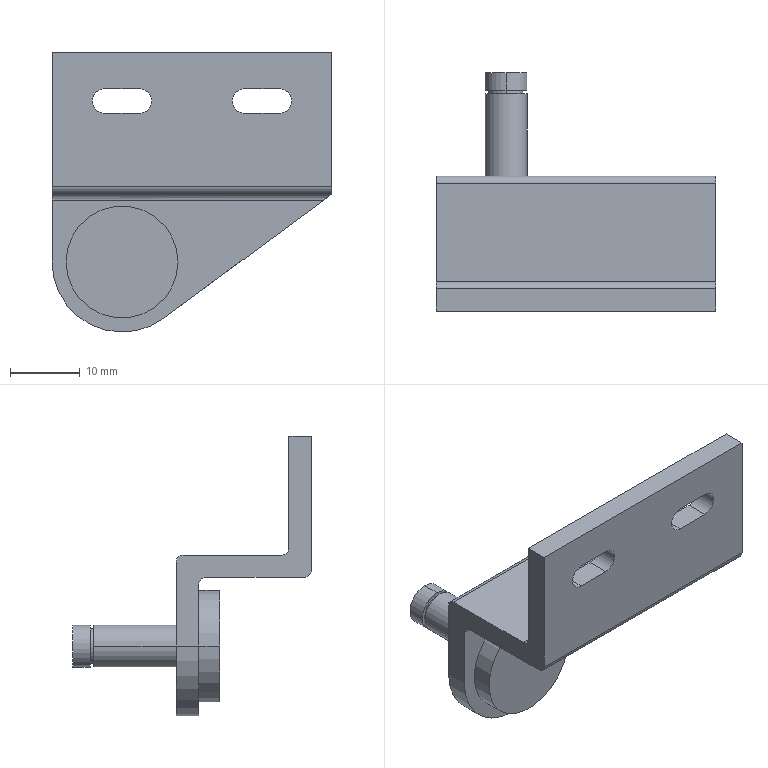Part | STEP file | Gas spring seat GSBR6C | 1 solid | 35 faces | box 40 x 34.1 x 40 mm | volume 7110 mm3 | plane 18 | cylinder 17 | commonest cylinder face diameters 2 x4 3.5 x4 6 x4 5 x2 16 x2 20 x1